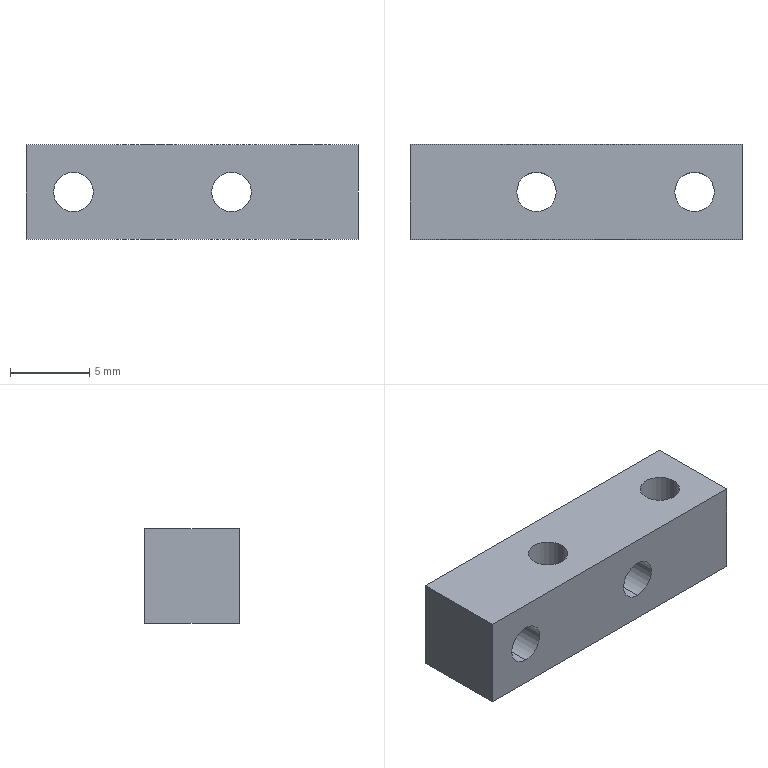Part | SolidWorks | features HoleWzd 2, Extrusion 1 | 1 solid | 14 faces | box 21 x 6 x 6 mm | volume 638.19 mm3 | cylinder 8 | plane 6 | commonest cylinder face diameters 2.5 x8
STEP:
#1=CARTESIAN_POINT('',(-7.5,0.,-1.25));
#2=VERTEX_POINT('',#1);
#3=CARTESIAN_POINT('',(-7.5,0.,1.25));
#4=VERTEX_POINT('',#3);
#5=CARTESIAN_POINT('',(-7.5,0.,0.));
#6=DIRECTION('',(0.,1.,0.));
#7=DIRECTION('',(0.,0.,1.));
#8=AXIS2_PLACEMENT_3D('',#5,#6,#7);
#9=CIRCLE('',#8,1.25);
#10=EDGE_CURVE('',#2,#4,#9,.T.);
#11=ORIENTED_EDGE('',*,*,#10,.F.);
#12=CARTESIAN_POINT('',(-7.5,6.,-1.25));
#13=VERTEX_POINT('',#12);
#14=CARTESIAN_POINT('',(-7.5,6.,-1.25));
#15=DIRECTION('',(0.,1.,0.));
#16=VECTOR('',#15,1000.);
#17=LINE('',#14,#16);
#18=EDGE_CURVE('',#2,#13,#17,.T.);
#19=ORIENTED_EDGE('',*,*,#18,.T.);
#20=CARTESIAN_POINT('',(-7.5,6.,1.25));
#21=VERTEX_POINT('',#20);
#22=CARTESIAN_POINT('',(-7.5,6.,0.));
#23=DIRECTION('',(0.,1.,0.));
#24=DIRECTION('',(0.,0.,1.));
#25=AXIS2_PLACEMENT_3D('',#22,#23,#24);
#26=CIRCLE('',#25,1.25);
#27=EDGE_CURVE('',#13,#21,#26,.T.);
#28=ORIENTED_EDGE('',*,*,#27,.T.);
#29=CARTESIAN_POINT('',(-7.5,6.,1.25));
#30=DIRECTION('',(0.,1.,0.));
#31=VECTOR('',#30,1000.);
#32=LINE('',#29,#31);
#33=EDGE_CURVE('',#4,#21,#32,.T.);
#34=ORIENTED_EDGE('',*,*,#33,.F.);
#35=EDGE_LOOP('',(#11,#19,#28,#34));
#36=FACE_OUTER_BOUND('',#35,.T.);
#37=CARTESIAN_POINT('',(-7.5,6.,0.));
#38=DIRECTION('',(0.,1.,0.));
#39=DIRECTION('',(0.,0.,1.));
#40=AXIS2_PLACEMENT_3D('',#37,#38,#39);
#41=CYLINDRICAL_SURFACE('',#40,1.25);
#42=ADVANCED_FACE('',(#36),#41,.F.);
#43=CARTESIAN_POINT('',(2.5,0.,-1.25));
#44=VERTEX_POINT('',#43);
#45=CARTESIAN_POINT('',(2.5,0.,1.25));
#46=VERTEX_POINT('',#45);
#47=CARTESIAN_POINT('',(2.5,0.,0.));
#48=DIRECTION('',(0.,1.,0.));
#49=DIRECTION('',(0.,0.,1.));
#50=AXIS2_PLACEMENT_3D('',#47,#48,#49);
#51=CIRCLE('',#50,1.25);
#52=EDGE_CURVE('',#44,#46,#51,.T.);
#53=ORIENTED_EDGE('',*,*,#52,.F.);
#54=CARTESIAN_POINT('',(2.5,6.,-1.25));
#55=VERTEX_POINT('',#54);
#56=CARTESIAN_POINT('',(2.5,6.,-1.25));
#57=DIRECTION('',(0.,1.,0.));
#58=VECTOR('',#57,1000.);
#59=LINE('',#56,#58);
#60=EDGE_CURVE('',#44,#55,#59,.T.);
#61=ORIENTED_EDGE('',*,*,#60,.T.);
#62=CARTESIAN_POINT('',(2.5,6.,1.25));
#63=VERTEX_POINT('',#62);
#64=CARTESIAN_POINT('',(2.5,6.,0.));
#65=DIRECTION('',(0.,1.,0.));
#66=DIRECTION('',(0.,0.,1.));
#67=AXIS2_PLACEMENT_3D('',#64,#65,#66);
#68=CIRCLE('',#67,1.25);
#69=EDGE_CURVE('',#55,#63,#68,.T.);
#70=ORIENTED_EDGE('',*,*,#69,.T.);
#71=CARTESIAN_POINT('',(2.5,6.,1.25));
#72=DIRECTION('',(0.,1.,0.));
#73=VECTOR('',#72,1000.);
#74=LINE('',#71,#73);
#75=EDGE_CURVE('',#46,#63,#74,.T.);
#76=ORIENTED_EDGE('',*,*,#75,.F.);
#77=EDGE_LOOP('',(#53,#61,#70,#76));
#78=FACE_OUTER_BOUND('',#77,.T.);
#79=CARTESIAN_POINT('',(2.5,6.,0.));
#80=DIRECTION('',(0.,1.,0.));
#81=DIRECTION('',(0.,0.,1.));
#82=AXIS2_PLACEMENT_3D('',#79,#80,#81);
#83=CYLINDRICAL_SURFACE('',#82,1.25);
#84=ADVANCED_FACE('',(#78),#83,.F.);
#85=CARTESIAN_POINT('',(6.25,3.,-3.));
#86=VERTEX_POINT('',#85);
#87=CARTESIAN_POINT('',(8.75,3.,-3.));
#88=VERTEX_POINT('',#87);
#89=CARTESIAN_POINT('',(7.5,3.,-3.));
#90=DIRECTION('',(0.,0.,1.));
#91=DIRECTION('',(1.,0.,0.));
#92=AXIS2_PLACEMENT_3D('',#89,#90,#91);
#93=CIRCLE('',#92,1.25);
#94=EDGE_CURVE('',#86,#88,#93,.T.);
#95=ORIENTED_EDGE('',*,*,#94,.F.);
#96=CARTESIAN_POINT('',(6.25,3.,3.));
#97=VERTEX_POINT('',#96);
#98=CARTESIAN_POINT('',(6.25,3.,3.));
#99=DIRECTION('',(0.,0.,1.));
#100=VECTOR('',#99,1000.);
#101=LINE('',#98,#100);
#102=EDGE_CURVE('',#86,#97,#101,.T.);
#103=ORIENTED_EDGE('',*,*,#102,.T.);
#104=CARTESIAN_POINT('',(8.75,3.,3.));
#105=VERTEX_POINT('',#104);
#106=CARTESIAN_POINT('',(7.5,3.,3.));
#107=DIRECTION('',(0.,0.,1.));
#108=DIRECTION('',(1.,0.,0.));
#109=AXIS2_PLACEMENT_3D('',#106,#107,#108);
#110=CIRCLE('',#109,1.25);
#111=EDGE_CURVE('',#97,#105,#110,.T.);
#112=ORIENTED_EDGE('',*,*,#111,.T.);
#113=CARTESIAN_POINT('',(8.75,3.,3.));
#114=DIRECTION('',(0.,0.,1.));
#115=VECTOR('',#114,1000.);
#116=LINE('',#113,#115);
#117=EDGE_CURVE('',#88,#105,#116,.T.);
#118=ORIENTED_EDGE('',*,*,#117,.F.);
#119=EDGE_LOOP('',(#95,#103,#112,#118));
#120=FACE_OUTER_BOUND('',#119,.T.);
#121=CARTESIAN_POINT('',(7.5,3.,3.));
#122=DIRECTION('',(0.,0.,1.));
#123=DIRECTION('',(1.,0.,0.));
#124=AXIS2_PLACEMENT_3D('',#121,#122,#123);
#125=CYLINDRICAL_SURFACE('',#124,1.25);
#126=ADVANCED_FACE('',(#120),#125,.F.);
#127=CARTESIAN_POINT('',(-3.75,3.,-3.));
#128=VERTEX_POINT('',#127);
#129=CARTESIAN_POINT('',(-1.25,3.,-3.));
#130=VERTEX_POINT('',#129);
#131=CARTESIAN_POINT('',(-2.5,3.,-3.));
#132=DIRECTION('',(0.,0.,1.));
#133=DIRECTION('',(1.,0.,0.));
#134=AXIS2_PLACEMENT_3D('',#131,#132,#133);
#135=CIRCLE('',#134,1.25);
#136=EDGE_CURVE('',#128,#130,#135,.T.);
#137=ORIENTED_EDGE('',*,*,#136,.F.);
#138=CARTESIAN_POINT('',(-3.75,3.,3.));
#139=VERTEX_POINT('',#138);
#140=CARTESIAN_POINT('',(-3.75,3.,3.));
#141=DIRECTION('',(0.,0.,1.));
#142=VECTOR('',#141,1000.);
#143=LINE('',#140,#142);
#144=EDGE_CURVE('',#128,#139,#143,.T.);
#145=ORIENTED_EDGE('',*,*,#144,.T.);
#146=CARTESIAN_POINT('',(-1.25,3.,3.));
#147=VERTEX_POINT('',#146);
#148=CARTESIAN_POINT('',(-2.5,3.,3.));
#149=DIRECTION('',(0.,0.,1.));
#150=DIRECTION('',(1.,0.,0.));
#151=AXIS2_PLACEMENT_3D('',#148,#149,#150);
#152=CIRCLE('',#151,1.25);
#153=EDGE_CURVE('',#139,#147,#152,.T.);
#154=ORIENTED_EDGE('',*,*,#153,.T.);
#155=CARTESIAN_POINT('',(-1.25,3.,3.));
#156=DIRECTION('',(0.,0.,1.));
#157=VECTOR('',#156,1000.);
#158=LINE('',#155,#157);
#159=EDGE_CURVE('',#130,#147,#158,.T.);
#160=ORIENTED_EDGE('',*,*,#159,.F.);
#161=EDGE_LOOP('',(#137,#145,#154,#160));
#162=FACE_OUTER_BOUND('',#161,.T.);
#163=CARTESIAN_POINT('',(-2.5,3.,3.));
#164=DIRECTION('',(0.,0.,1.));
#165=DIRECTION('',(1.,0.,0.));
#166=AXIS2_PLACEMENT_3D('',#163,#164,#165);
#167=CYLINDRICAL_SURFACE('',#166,1.25);
#168=ADVANCED_FACE('',(#162),#167,.F.);
#169=CARTESIAN_POINT('',(-10.5,0.,-3.));
#170=VERTEX_POINT('',#169);
#171=CARTESIAN_POINT('',(-10.5,0.,3.));
#172=VERTEX_POINT('',#171);
#173=CARTESIAN_POINT('',(-10.5,0.,3.));
#174=DIRECTION('',(0.,0.,1.));
#175=VECTOR('',#174,1000.);
#176=LINE('',#173,#175);
#177=EDGE_CURVE('',#170,#172,#176,.T.);
#178=ORIENTED_EDGE('',*,*,#177,.T.);
#179=CARTESIAN_POINT('',(-10.5,6.,3.));
#180=VERTEX_POINT('',#179);
#181=CARTESIAN_POINT('',(-10.5,6.,3.));
#182=DIRECTION('',(0.,-1.,0.));
#183=VECTOR('',#182,1000.);
#184=LINE('',#181,#183);
#185=EDGE_CURVE('',#180,#172,#184,.T.);
#186=ORIENTED_EDGE('',*,*,#185,.F.);
#187=CARTESIAN_POINT('',(-10.5,6.,-3.));
#188=VERTEX_POINT('',#187);
#189=CARTESIAN_POINT('',(-10.5,6.,3.));
#190=DIRECTION('',(0.,0.,1.));
#191=VECTOR('',#190,1000.);
#192=LINE('',#189,#191);
#193=EDGE_CURVE('',#188,#180,#192,.T.);
#194=ORIENTED_EDGE('',*,*,#193,.F.);
#195=CARTESIAN_POINT('',(-10.5,6.,-3.));
#196=DIRECTION('',(0.,-1.,0.));
#197=VECTOR('',#196,1000.);
#198=LINE('',#195,#197);
#199=EDGE_CURVE('',#188,#170,#198,.T.);
#200=ORIENTED_EDGE('',*,*,#199,.T.);
#201=EDGE_LOOP('',(#178,#186,#194,#200));
#202=FACE_OUTER_BOUND('',#201,.T.);
#203=CARTESIAN_POINT('',(-10.5,6.,3.));
#204=DIRECTION('',(1.,0.,0.));
#205=DIRECTION('',(0.,0.,-1.));
#206=AXIS2_PLACEMENT_3D('',#203,#204,#205);
#207=PLANE('',#206);
#208=ADVANCED_FACE('',(#202),#207,.F.);
#209=CARTESIAN_POINT('',(7.5,3.,3.));
#210=DIRECTION('',(0.,0.,1.));
#211=DIRECTION('',(1.,0.,0.));
#212=AXIS2_PLACEMENT_3D('',#209,#210,#211);
#213=CIRCLE('',#212,1.25);
#214=EDGE_CURVE('',#105,#97,#213,.T.);
#215=ORIENTED_EDGE('',*,*,#214,.F.);
#216=ORIENTED_EDGE('',*,*,#111,.F.);
#217=EDGE_LOOP('',(#215,#216));
#218=FACE_BOUND('',#217,.T.);
#219=CARTESIAN_POINT('',(-2.5,3.,3.));
#220=DIRECTION('',(0.,0.,1.));
#221=DIRECTION('',(1.,0.,0.));
#222=AXIS2_PLACEMENT_3D('',#219,#220,#221);
#223=CIRCLE('',#222,1.25);
#224=EDGE_CURVE('',#147,#139,#223,.T.);
#225=ORIENTED_EDGE('',*,*,#224,.F.);
#226=ORIENTED_EDGE('',*,*,#153,.F.);
#227=EDGE_LOOP('',(#225,#226));
#228=FACE_BOUND('',#227,.T.);
#229=CARTESIAN_POINT('',(10.5,0.,3.));
#230=VERTEX_POINT('',#229);
#231=CARTESIAN_POINT('',(10.5,0.,3.));
#232=DIRECTION('',(1.,0.,0.));
#233=VECTOR('',#232,1000.);
#234=LINE('',#231,#233);
#235=EDGE_CURVE('',#172,#230,#234,.T.);
#236=ORIENTED_EDGE('',*,*,#235,.T.);
#237=CARTESIAN_POINT('',(10.5,6.,3.));
#238=VERTEX_POINT('',#237);
#239=CARTESIAN_POINT('',(10.5,6.,3.));
#240=DIRECTION('',(0.,-1.,0.));
#241=VECTOR('',#240,1000.);
#242=LINE('',#239,#241);
#243=EDGE_CURVE('',#238,#230,#242,.T.);
#244=ORIENTED_EDGE('',*,*,#243,.F.);
#245=CARTESIAN_POINT('',(10.5,6.,3.));
#246=DIRECTION('',(1.,0.,0.));
#247=VECTOR('',#246,1000.);
#248=LINE('',#245,#247);
#249=EDGE_CURVE('',#180,#238,#248,.T.);
#250=ORIENTED_EDGE('',*,*,#249,.F.);
#251=ORIENTED_EDGE('',*,*,#185,.T.);
#252=EDGE_LOOP('',(#236,#244,#250,#251));
#253=FACE_OUTER_BOUND('',#252,.T.);
#254=CARTESIAN_POINT('',(10.5,6.,3.));
#255=DIRECTION('',(0.,0.,-1.));
#256=DIRECTION('',(-1.,0.,0.));
#257=AXIS2_PLACEMENT_3D('',#254,#255,#256);
#258=PLANE('',#257);
#259=ADVANCED_FACE('',(#218,#228,#253),#258,.F.);
#260=CARTESIAN_POINT('',(10.5,0.,-3.));
#261=VERTEX_POINT('',#260);
#262=CARTESIAN_POINT('',(10.5,0.,3.));
#263=DIRECTION('',(0.,0.,-1.));
#264=VECTOR('',#263,1000.);
#265=LINE('',#262,#264);
#266=EDGE_CURVE('',#230,#261,#265,.T.);
#267=ORIENTED_EDGE('',*,*,#266,.T.);
#268=CARTESIAN_POINT('',(10.5,6.,-3.));
#269=VERTEX_POINT('',#268);
#270=CARTESIAN_POINT('',(10.5,6.,-3.));
#271=DIRECTION('',(0.,-1.,0.));
#272=VECTOR('',#271,1000.);
#273=LINE('',#270,#272);
#274=EDGE_CURVE('',#269,#261,#273,.T.);
#275=ORIENTED_EDGE('',*,*,#274,.F.);
#276=CARTESIAN_POINT('',(10.5,6.,3.));
#277=DIRECTION('',(0.,0.,-1.));
#278=VECTOR('',#277,1000.);
#279=LINE('',#276,#278);
#280=EDGE_CURVE('',#238,#269,#279,.T.);
#281=ORIENTED_EDGE('',*,*,#280,.F.);
#282=ORIENTED_EDGE('',*,*,#243,.T.);
#283=EDGE_LOOP('',(#267,#275,#281,#282));
#284=FACE_OUTER_BOUND('',#283,.T.);
#285=CARTESIAN_POINT('',(10.5,6.,3.));
#286=DIRECTION('',(-1.,0.,0.));
#287=DIRECTION('',(0.,0.,1.));
#288=AXIS2_PLACEMENT_3D('',#285,#286,#287);
#289=PLANE('',#288);
#290=ADVANCED_FACE('',(#284),#289,.F.);
#291=CARTESIAN_POINT('',(7.5,3.,-3.));
#292=DIRECTION('',(0.,0.,1.));
#293=DIRECTION('',(1.,0.,0.));
#294=AXIS2_PLACEMENT_3D('',#291,#292,#293);
#295=CIRCLE('',#294,1.25);
#296=EDGE_CURVE('',#88,#86,#295,.T.);
#297=ORIENTED_EDGE('',*,*,#296,.T.);
#298=ORIENTED_EDGE('',*,*,#94,.T.);
#299=EDGE_LOOP('',(#297,#298));
#300=FACE_BOUND('',#299,.T.);
#301=CARTESIAN_POINT('',(-2.5,3.,-3.));
#302=DIRECTION('',(0.,0.,1.));
#303=DIRECTION('',(1.,0.,0.));
#304=AXIS2_PLACEMENT_3D('',#301,#302,#303);
#305=CIRCLE('',#304,1.25);
#306=EDGE_CURVE('',#130,#128,#305,.T.);
#307=ORIENTED_EDGE('',*,*,#306,.T.);
#308=ORIENTED_EDGE('',*,*,#136,.T.);
#309=EDGE_LOOP('',(#307,#308));
#310=FACE_BOUND('',#309,.T.);
#311=CARTESIAN_POINT('',(10.5,0.,-3.));
#312=DIRECTION('',(-1.,0.,0.));
#313=VECTOR('',#312,1000.);
#314=LINE('',#311,#313);
#315=EDGE_CURVE('',#261,#170,#314,.T.);
#316=ORIENTED_EDGE('',*,*,#315,.T.);
#317=ORIENTED_EDGE('',*,*,#199,.F.);
#318=CARTESIAN_POINT('',(10.5,6.,-3.));
#319=DIRECTION('',(-1.,0.,0.));
#320=VECTOR('',#319,1000.);
#321=LINE('',#318,#320);
#322=EDGE_CURVE('',#269,#188,#321,.T.);
#323=ORIENTED_EDGE('',*,*,#322,.F.);
#324=ORIENTED_EDGE('',*,*,#274,.T.);
#325=EDGE_LOOP('',(#316,#317,#323,#324));
#326=FACE_OUTER_BOUND('',#325,.T.);
#327=CARTESIAN_POINT('',(10.5,6.,-3.));
#328=DIRECTION('',(0.,0.,1.));
#329=DIRECTION('',(1.,0.,0.));
#330=AXIS2_PLACEMENT_3D('',#327,#328,#329);
#331=PLANE('',#330);
#332=ADVANCED_FACE('',(#300,#310,#326),#331,.F.);
#333=CARTESIAN_POINT('',(-7.5,6.,0.));
#334=DIRECTION('',(0.,1.,0.));
#335=DIRECTION('',(0.,0.,1.));
#336=AXIS2_PLACEMENT_3D('',#333,#334,#335);
#337=CIRCLE('',#336,1.25);
#338=EDGE_CURVE('',#21,#13,#337,.T.);
#339=ORIENTED_EDGE('',*,*,#338,.F.);
#340=ORIENTED_EDGE('',*,*,#27,.F.);
#341=EDGE_LOOP('',(#339,#340));
#342=FACE_BOUND('',#341,.T.);
#343=CARTESIAN_POINT('',(2.5,6.,0.));
#344=DIRECTION('',(0.,1.,0.));
#345=DIRECTION('',(0.,0.,1.));
#346=AXIS2_PLACEMENT_3D('',#343,#344,#345);
#347=CIRCLE('',#346,1.25);
#348=EDGE_CURVE('',#63,#55,#347,.T.);
#349=ORIENTED_EDGE('',*,*,#348,.F.);
#350=ORIENTED_EDGE('',*,*,#69,.F.);
#351=EDGE_LOOP('',(#349,#350));
#352=FACE_BOUND('',#351,.T.);
#353=ORIENTED_EDGE('',*,*,#193,.T.);
#354=ORIENTED_EDGE('',*,*,#249,.T.);
#355=ORIENTED_EDGE('',*,*,#280,.T.);
#356=ORIENTED_EDGE('',*,*,#322,.T.);
#357=EDGE_LOOP('',(#353,#354,#355,#356));
#358=FACE_OUTER_BOUND('',#357,.T.);
#359=CARTESIAN_POINT('',(0.,6.,0.));
#360=DIRECTION('',(0.,1.,0.));
#361=DIRECTION('',(0.,0.,1.));
#362=AXIS2_PLACEMENT_3D('',#359,#360,#361);
#363=PLANE('',#362);
#364=ADVANCED_FACE('',(#342,#352,#358),#363,.T.);
#365=CARTESIAN_POINT('',(-7.5,0.,0.));
#366=DIRECTION('',(0.,1.,0.));
#367=DIRECTION('',(0.,0.,1.));
#368=AXIS2_PLACEMENT_3D('',#365,#366,#367);
#369=CIRCLE('',#368,1.25);
#370=EDGE_CURVE('',#4,#2,#369,.T.);
#371=ORIENTED_EDGE('',*,*,#370,.T.);
#372=ORIENTED_EDGE('',*,*,#10,.T.);
#373=EDGE_LOOP('',(#371,#372));
#374=FACE_BOUND('',#373,.T.);
#375=CARTESIAN_POINT('',(2.5,0.,0.));
#376=DIRECTION('',(0.,1.,0.));
#377=DIRECTION('',(0.,0.,1.));
#378=AXIS2_PLACEMENT_3D('',#375,#376,#377);
#379=CIRCLE('',#378,1.25);
#380=EDGE_CURVE('',#46,#44,#379,.T.);
#381=ORIENTED_EDGE('',*,*,#380,.T.);
#382=ORIENTED_EDGE('',*,*,#52,.T.);
#383=EDGE_LOOP('',(#381,#382));
#384=FACE_BOUND('',#383,.T.);
#385=ORIENTED_EDGE('',*,*,#177,.F.);
#386=ORIENTED_EDGE('',*,*,#315,.F.);
#387=ORIENTED_EDGE('',*,*,#266,.F.);
#388=ORIENTED_EDGE('',*,*,#235,.F.);
#389=EDGE_LOOP('',(#385,#386,#387,#388));
#390=FACE_OUTER_BOUND('',#389,.T.);
#391=CARTESIAN_POINT('',(0.,0.,0.));
#392=DIRECTION('',(0.,1.,0.));
#393=DIRECTION('',(0.,0.,1.));
#394=AXIS2_PLACEMENT_3D('',#391,#392,#393);
#395=PLANE('',#394);
#396=ADVANCED_FACE('',(#374,#384,#390),#395,.F.);
#397=ORIENTED_EDGE('',*,*,#144,.F.);
#398=ORIENTED_EDGE('',*,*,#306,.F.);
#399=ORIENTED_EDGE('',*,*,#159,.T.);
#400=ORIENTED_EDGE('',*,*,#224,.T.);
#401=EDGE_LOOP('',(#397,#398,#399,#400));
#402=FACE_OUTER_BOUND('',#401,.T.);
#403=CARTESIAN_POINT('',(-2.5,3.,3.));
#404=DIRECTION('',(0.,0.,1.));
#405=DIRECTION('',(1.,0.,0.));
#406=AXIS2_PLACEMENT_3D('',#403,#404,#405);
#407=CYLINDRICAL_SURFACE('',#406,1.25);
#408=ADVANCED_FACE('',(#402),#407,.F.);
#409=ORIENTED_EDGE('',*,*,#102,.F.);
#410=ORIENTED_EDGE('',*,*,#296,.F.);
#411=ORIENTED_EDGE('',*,*,#117,.T.);
#412=ORIENTED_EDGE('',*,*,#214,.T.);
#413=EDGE_LOOP('',(#409,#410,#411,#412));
#414=FACE_OUTER_BOUND('',#413,.T.);
#415=CARTESIAN_POINT('',(7.5,3.,3.));
#416=DIRECTION('',(0.,0.,1.));
#417=DIRECTION('',(1.,0.,0.));
#418=AXIS2_PLACEMENT_3D('',#415,#416,#417);
#419=CYLINDRICAL_SURFACE('',#418,1.25);
#420=ADVANCED_FACE('',(#414),#419,.F.);
#421=ORIENTED_EDGE('',*,*,#60,.F.);
#422=ORIENTED_EDGE('',*,*,#380,.F.);
#423=ORIENTED_EDGE('',*,*,#75,.T.);
#424=ORIENTED_EDGE('',*,*,#348,.T.);
#425=EDGE_LOOP('',(#421,#422,#423,#424));
#426=FACE_OUTER_BOUND('',#425,.T.);
#427=CARTESIAN_POINT('',(2.5,6.,0.));
#428=DIRECTION('',(0.,1.,0.));
#429=DIRECTION('',(0.,0.,1.));
#430=AXIS2_PLACEMENT_3D('',#427,#428,#429);
#431=CYLINDRICAL_SURFACE('',#430,1.25);
#432=ADVANCED_FACE('',(#426),#431,.F.);
#433=ORIENTED_EDGE('',*,*,#18,.F.);
#434=ORIENTED_EDGE('',*,*,#370,.F.);
#435=ORIENTED_EDGE('',*,*,#33,.T.);
#436=ORIENTED_EDGE('',*,*,#338,.T.);
#437=EDGE_LOOP('',(#433,#434,#435,#436));
#438=FACE_OUTER_BOUND('',#437,.T.);
#439=CARTESIAN_POINT('',(-7.5,6.,0.));
#440=DIRECTION('',(0.,1.,0.));
#441=DIRECTION('',(0.,0.,1.));
#442=AXIS2_PLACEMENT_3D('',#439,#440,#441);
#443=CYLINDRICAL_SURFACE('',#442,1.25);
#444=ADVANCED_FACE('',(#438),#443,.F.);
#445=CLOSED_SHELL('',(#42,#84,#126,#168,#208,#259,#290,#332,#364,#396,#408,#420,#432,#444));
#446=MANIFOLD_SOLID_BREP('',#445);
#447=CARTESIAN_POINT('',(0.,0.,0.));
#448=DIRECTION('',(0.,0.,1.));
#449=DIRECTION('',(1.,0.,0.));
#450=AXIS2_PLACEMENT_3D('',#447,#448,#449);
#451=(LENGTH_UNIT()NAMED_UNIT(*)SI_UNIT(.MILLI.,.METRE.));
#452=UNCERTAINTY_MEASURE_WITH_UNIT(LENGTH_MEASURE(0.00001),#451,'','');
#453=(NAMED_UNIT(*)PLANE_ANGLE_UNIT()SI_UNIT($,.RADIAN.));
#454=(NAMED_UNIT(*)SI_UNIT($,.STERADIAN.)SOLID_ANGLE_UNIT());
#455=(GEOMETRIC_REPRESENTATION_CONTEXT(3)GLOBAL_UNCERTAINTY_ASSIGNED_CONTEXT((#452))GLOBAL_UNIT_ASSIGNED_CONTEXT((#451,#453,#454))REPRESENTATION_CONTEXT('',''));
#456=ADVANCED_BREP_SHAPE_REPRESENTATION('',(#446,#450),#455);